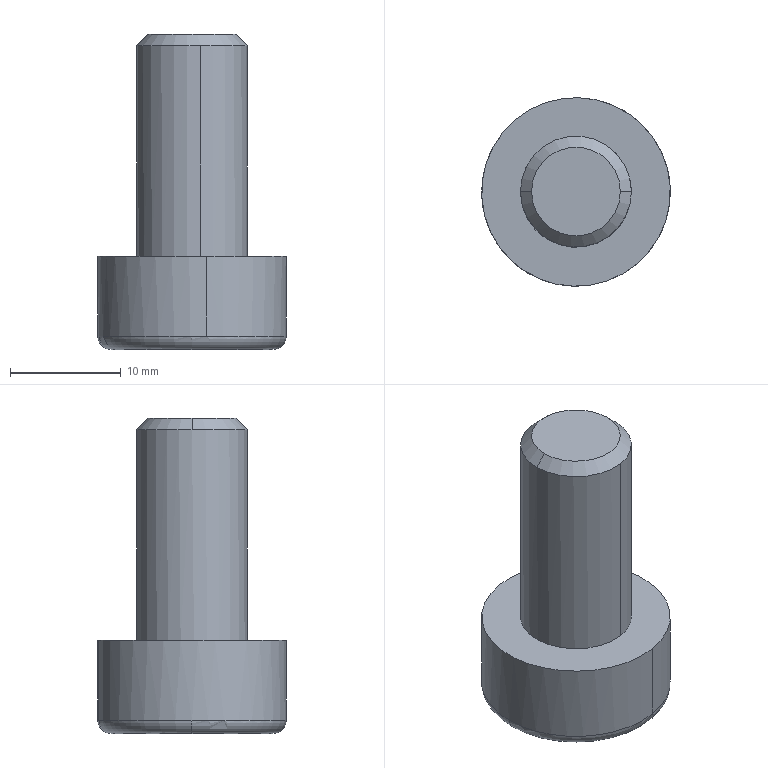Part | SolidWorks | features BaseBody 1 | 1 solid | 18 faces | box 17.001 x 17 x 28.402 mm | volume 3098 mm3 | plane 10 | cylinder 4 | cone 2 | torus 2 | commonest cylinder face diameters 10 x2 17 x2
STEP:
#1=CARTESIAN_POINT('',(410.058,334.317,39.477));
#2=VERTEX_POINT('',#1);
#3=CARTESIAN_POINT('',(402.058,334.317,39.476));
#4=VERTEX_POINT('',#3);
#5=CARTESIAN_POINT('',(406.058,334.317,39.477));
#6=DIRECTION('',(-0.0001435,-0.000000521,1.));
#7=DIRECTION('',(-1.,0.,-0.0001435));
#8=AXIS2_PLACEMENT_3D('',#5,#6,#7);
#9=CIRCLE('',#8,4.);
#10=EDGE_CURVE('',#2,#4,#9,.T.);
#11=ORIENTED_EDGE('',*,*,#10,.F.);
#12=CARTESIAN_POINT('',(411.058,334.317,38.477));
#13=VERTEX_POINT('',#12);
#14=CARTESIAN_POINT('',(410.558,334.317,38.977));
#15=DIRECTION('',(0.7072,0.000000369,-0.707));
#16=VECTOR('',#15,1000.);
#17=LINE('',#14,#16);
#18=EDGE_CURVE('',#2,#13,#17,.T.);
#19=ORIENTED_EDGE('',*,*,#18,.T.);
#20=CARTESIAN_POINT('',(405.284,339.257,38.477));
#21=VERTEX_POINT('',#20);
#22=CARTESIAN_POINT('',(406.058,334.317,38.477));
#23=DIRECTION('',(-0.0001435,-0.000000521,1.));
#24=DIRECTION('',(-0.1548,0.988,-0.00002169));
#25=AXIS2_PLACEMENT_3D('',#22,#23,#24);
#26=CIRCLE('',#25,5.);
#27=EDGE_CURVE('',#13,#21,#26,.T.);
#28=ORIENTED_EDGE('',*,*,#27,.T.);
#29=CARTESIAN_POINT('',(401.058,334.317,38.476));
#30=VERTEX_POINT('',#29);
#31=CARTESIAN_POINT('',(406.058,334.317,38.477));
#32=DIRECTION('',(-0.0001435,-0.000000521,1.));
#33=DIRECTION('',(-0.1548,0.988,-0.00002169));
#34=AXIS2_PLACEMENT_3D('',#31,#32,#33);
#35=CIRCLE('',#34,5.);
#36=EDGE_CURVE('',#21,#30,#35,.T.);
#37=ORIENTED_EDGE('',*,*,#36,.T.);
#38=CARTESIAN_POINT('',(401.558,334.317,38.976));
#39=DIRECTION('',(-0.707,0.000000369,-0.7072));
#40=VECTOR('',#39,1000.);
#41=LINE('',#38,#40);
#42=EDGE_CURVE('',#4,#30,#41,.T.);
#43=ORIENTED_EDGE('',*,*,#42,.F.);
#44=EDGE_LOOP('',(#11,#19,#28,#37,#43));
#45=FACE_OUTER_BOUND('',#44,.T.);
#46=CARTESIAN_POINT('',(406.058,334.317,38.977));
#47=DIRECTION('',(0.0001435,0.000000521,-1.));
#48=DIRECTION('',(-1.,0.,-0.0001435));
#49=AXIS2_PLACEMENT_3D('',#46,#47,#48);
#50=CONICAL_SURFACE('',#49,4.5,0.7854);
#51=ADVANCED_FACE('',(#45),#50,.T.);
#52=CARTESIAN_POINT('',(406.835,329.377,19.477));
#53=VERTEX_POINT('',#52);
#54=CARTESIAN_POINT('',(405.287,339.257,19.477));
#55=VERTEX_POINT('',#54);
#56=CARTESIAN_POINT('',(406.061,334.317,19.477));
#57=DIRECTION('',(0.0001435,0.000000521,-1.));
#58=DIRECTION('',(1.,0.,0.0001435));
#59=AXIS2_PLACEMENT_3D('',#56,#57,#58);
#60=CIRCLE('',#59,5.);
#61=EDGE_CURVE('',#53,#55,#60,.T.);
#62=ORIENTED_EDGE('',*,*,#61,.F.);
#63=CARTESIAN_POINT('',(406.832,329.377,38.477));
#64=VERTEX_POINT('',#63);
#65=CARTESIAN_POINT('',(406.832,329.377,41.277));
#66=DIRECTION('',(-0.0001435,-0.000000521,1.));
#67=VECTOR('',#66,1000.);
#68=LINE('',#65,#67);
#69=EDGE_CURVE('',#53,#64,#68,.T.);
#70=ORIENTED_EDGE('',*,*,#69,.T.);
#71=CARTESIAN_POINT('',(406.058,334.317,38.477));
#72=DIRECTION('',(-0.0001435,-0.000000521,1.));
#73=DIRECTION('',(-0.1548,0.988,-0.00002169));
#74=AXIS2_PLACEMENT_3D('',#71,#72,#73);
#75=CIRCLE('',#74,5.);
#76=EDGE_CURVE('',#30,#64,#75,.T.);
#77=ORIENTED_EDGE('',*,*,#76,.F.);
#78=ORIENTED_EDGE('',*,*,#36,.F.);
#79=CARTESIAN_POINT('',(405.284,339.257,41.277));
#80=DIRECTION('',(-0.0001435,-0.000000521,1.));
#81=VECTOR('',#80,1000.);
#82=LINE('',#79,#81);
#83=EDGE_CURVE('',#55,#21,#82,.T.);
#84=ORIENTED_EDGE('',*,*,#83,.F.);
#85=EDGE_LOOP('',(#62,#70,#77,#78,#84));
#86=FACE_OUTER_BOUND('',#85,.T.);
#87=CARTESIAN_POINT('',(406.058,334.317,41.277));
#88=DIRECTION('',(-0.0001435,-0.000000521,1.));
#89=DIRECTION('',(-0.1548,0.988,-0.00002169));
#90=AXIS2_PLACEMENT_3D('',#87,#88,#89);
#91=CYLINDRICAL_SURFACE('',#90,5.);
#92=ADVANCED_FACE('',(#86),#91,.T.);
#93=CARTESIAN_POINT('',(404.747,342.715,19.476));
#94=VERTEX_POINT('',#93);
#95=CARTESIAN_POINT('',(407.378,325.919,19.477));
#96=VERTEX_POINT('',#95);
#97=CARTESIAN_POINT('',(406.062,334.317,19.477));
#98=DIRECTION('',(-0.0001435,-0.000000521,1.));
#99=DIRECTION('',(-0.1548,0.988,-0.00002169));
#100=AXIS2_PLACEMENT_3D('',#97,#98,#99);
#101=CIRCLE('',#100,8.5);
#102=EDGE_CURVE('',#94,#96,#101,.T.);
#103=ORIENTED_EDGE('',*,*,#102,.F.);
#104=CARTESIAN_POINT('',(404.748,342.715,12.276));
#105=VERTEX_POINT('',#104);
#106=CARTESIAN_POINT('',(404.747,342.715,19.476));
#107=DIRECTION('',(0.0001435,0.000000521,-1.));
#108=VECTOR('',#107,1000.);
#109=LINE('',#106,#108);
#110=EDGE_CURVE('',#94,#105,#109,.T.);
#111=ORIENTED_EDGE('',*,*,#110,.T.);
#112=CARTESIAN_POINT('',(397.563,334.317,12.275));
#113=VERTEX_POINT('',#112);
#114=CARTESIAN_POINT('',(406.063,334.317,12.277));
#115=DIRECTION('',(0.0001435,0.000000521,-1.));
#116=DIRECTION('',(-0.1548,0.988,-0.00002169));
#117=AXIS2_PLACEMENT_3D('',#114,#115,#116);
#118=CIRCLE('',#117,8.5);
#119=EDGE_CURVE('',#113,#105,#118,.T.);
#120=ORIENTED_EDGE('',*,*,#119,.F.);
#121=CARTESIAN_POINT('',(407.379,325.919,12.277));
#122=VERTEX_POINT('',#121);
#123=CARTESIAN_POINT('',(406.063,334.317,12.277));
#124=DIRECTION('',(0.0001435,0.000000521,-1.));
#125=DIRECTION('',(-0.1548,0.988,-0.00002169));
#126=AXIS2_PLACEMENT_3D('',#123,#124,#125);
#127=CIRCLE('',#126,8.5);
#128=EDGE_CURVE('',#122,#113,#127,.T.);
#129=ORIENTED_EDGE('',*,*,#128,.F.);
#130=CARTESIAN_POINT('',(407.378,325.919,19.477));
#131=DIRECTION('',(0.0001435,0.000000521,-1.));
#132=VECTOR('',#131,1000.);
#133=LINE('',#130,#132);
#134=EDGE_CURVE('',#96,#122,#133,.T.);
#135=ORIENTED_EDGE('',*,*,#134,.F.);
#136=EDGE_LOOP('',(#103,#111,#120,#129,#135));
#137=FACE_OUTER_BOUND('',#136,.T.);
#138=CARTESIAN_POINT('',(406.062,334.317,19.477));
#139=DIRECTION('',(0.0001435,0.000000521,-1.));
#140=DIRECTION('',(0.1548,-0.988,0.00002169));
#141=AXIS2_PLACEMENT_3D('',#138,#139,#140);
#142=CYLINDRICAL_SURFACE('',#141,8.5);
#143=ADVANCED_FACE('',(#137),#142,.T.);
#144=ORIENTED_EDGE('',*,*,#119,.T.);
#145=CARTESIAN_POINT('',(414.563,334.317,12.278));
#146=VERTEX_POINT('',#145);
#147=CARTESIAN_POINT('',(406.063,334.317,12.277));
#148=DIRECTION('',(0.0001435,0.000000521,-1.));
#149=DIRECTION('',(-0.1548,0.988,-0.00002169));
#150=AXIS2_PLACEMENT_3D('',#147,#148,#149);
#151=CIRCLE('',#150,8.5);
#152=EDGE_CURVE('',#105,#146,#151,.T.);
#153=ORIENTED_EDGE('',*,*,#152,.T.);
#154=CARTESIAN_POINT('',(413.364,334.317,11.078));
#155=VERTEX_POINT('',#154);
#156=CARTESIAN_POINT('',(413.363,334.317,12.278));
#157=DIRECTION('',(0.,1.,0.000000521));
#158=DIRECTION('',(0.,-0.000000521,1.));
#159=AXIS2_PLACEMENT_3D('',#156,#157,#158);
#160=CIRCLE('',#159,1.2);
#161=EDGE_CURVE('',#146,#155,#160,.T.);
#162=ORIENTED_EDGE('',*,*,#161,.T.);
#163=CARTESIAN_POINT('',(398.764,334.317,11.076));
#164=VERTEX_POINT('',#163);
#165=CARTESIAN_POINT('',(406.064,334.317,11.077));
#166=DIRECTION('',(0.0001435,0.000000521,-1.));
#167=DIRECTION('',(-1.,0.,-0.0001435));
#168=AXIS2_PLACEMENT_3D('',#165,#166,#167);
#169=CIRCLE('',#168,7.3);
#170=EDGE_CURVE('',#164,#155,#169,.T.);
#171=ORIENTED_EDGE('',*,*,#170,.F.);
#172=CARTESIAN_POINT('',(398.763,334.317,12.276));
#173=DIRECTION('',(0.,-1.,-0.000000521));
#174=DIRECTION('',(0.,0.000000521,-1.));
#175=AXIS2_PLACEMENT_3D('',#172,#173,#174);
#176=CIRCLE('',#175,1.2);
#177=EDGE_CURVE('',#113,#164,#176,.T.);
#178=ORIENTED_EDGE('',*,*,#177,.F.);
#179=EDGE_LOOP('',(#144,#153,#162,#171,#178));
#180=FACE_OUTER_BOUND('',#179,.T.);
#181=CARTESIAN_POINT('',(406.063,334.317,12.277));
#182=DIRECTION('',(0.0001435,0.000000521,-1.));
#183=DIRECTION('',(-1.,0.,-0.0001435));
#184=AXIS2_PLACEMENT_3D('',#181,#182,#183);
#185=TOROIDAL_SURFACE('',#184,7.3,1.2);
#186=ADVANCED_FACE('',(#180),#185,.T.);
#187=CARTESIAN_POINT('',(410.797,335.039,17.077));
#188=VERTEX_POINT('',#187);
#189=CARTESIAN_POINT('',(409.094,330.624,17.077));
#190=VERTEX_POINT('',#189);
#191=CARTESIAN_POINT('',(410.797,335.039,17.077));
#192=DIRECTION('',(-0.3599,-0.933,-0.00005213));
#193=VECTOR('',#192,1000.);
#194=LINE('',#191,#193);
#195=EDGE_CURVE('',#188,#190,#194,.T.);
#196=ORIENTED_EDGE('',*,*,#195,.T.);
#197=CARTESIAN_POINT('',(404.419,329.891,17.076));
#198=VERTEX_POINT('',#197);
#199=CARTESIAN_POINT('',(409.094,330.624,17.077));
#200=DIRECTION('',(-0.988,-0.1548,-0.0001418));
#201=VECTOR('',#200,1000.);
#202=LINE('',#199,#201);
#203=EDGE_CURVE('',#190,#198,#202,.T.);
#204=ORIENTED_EDGE('',*,*,#203,.T.);
#205=CARTESIAN_POINT('',(401.447,333.574,17.076));
#206=VERTEX_POINT('',#205);
#207=CARTESIAN_POINT('',(404.419,329.891,17.076));
#208=DIRECTION('',(-0.628,0.7782,-0.0000897));
#209=VECTOR('',#208,1000.);
#210=LINE('',#207,#209);
#211=EDGE_CURVE('',#198,#206,#210,.T.);
#212=ORIENTED_EDGE('',*,*,#211,.T.);
#213=CARTESIAN_POINT('',(403.15,337.989,17.076));
#214=VERTEX_POINT('',#213);
#215=CARTESIAN_POINT('',(401.447,333.574,17.076));
#216=DIRECTION('',(0.3599,0.933,0.00005213));
#217=VECTOR('',#216,1000.);
#218=LINE('',#215,#217);
#219=EDGE_CURVE('',#206,#214,#218,.T.);
#220=ORIENTED_EDGE('',*,*,#219,.T.);
#221=CARTESIAN_POINT('',(407.825,338.721,17.077));
#222=VERTEX_POINT('',#221);
#223=CARTESIAN_POINT('',(403.15,337.989,17.076));
#224=DIRECTION('',(0.988,0.1548,0.0001418));
#225=VECTOR('',#224,1000.);
#226=LINE('',#223,#225);
#227=EDGE_CURVE('',#214,#222,#226,.T.);
#228=ORIENTED_EDGE('',*,*,#227,.T.);
#229=CARTESIAN_POINT('',(407.825,338.721,17.077));
#230=DIRECTION('',(0.628,-0.7782,0.0000897));
#231=VECTOR('',#230,1000.);
#232=LINE('',#229,#231);
#233=EDGE_CURVE('',#222,#188,#232,.T.);
#234=ORIENTED_EDGE('',*,*,#233,.T.);
#235=EDGE_LOOP('',(#196,#204,#212,#220,#228,#234));
#236=FACE_OUTER_BOUND('',#235,.T.);
#237=CARTESIAN_POINT('',(410.567,305.568,17.077));
#238=DIRECTION('',(0.0001435,0.000000521,-1.));
#239=DIRECTION('',(0.,-1.,-0.000000521));
#240=AXIS2_PLACEMENT_3D('',#237,#238,#239);
#241=PLANE('',#240);
#242=ADVANCED_FACE('',(#236),#241,.T.);
#243=CARTESIAN_POINT('',(409.095,330.624,11.077));
#244=VERTEX_POINT('',#243);
#245=CARTESIAN_POINT('',(409.094,330.624,17.077));
#246=DIRECTION('',(0.0001435,0.000000521,-1.));
#247=VECTOR('',#246,1000.);
#248=LINE('',#245,#247);
#249=EDGE_CURVE('',#190,#244,#248,.T.);
#250=ORIENTED_EDGE('',*,*,#249,.F.);
#251=ORIENTED_EDGE('',*,*,#195,.F.);
#252=CARTESIAN_POINT('',(410.798,335.039,11.077));
#253=VERTEX_POINT('',#252);
#254=CARTESIAN_POINT('',(410.797,335.039,17.077));
#255=DIRECTION('',(0.0001435,0.000000521,-1.));
#256=VECTOR('',#255,1000.);
#257=LINE('',#254,#256);
#258=EDGE_CURVE('',#188,#253,#257,.T.);
#259=ORIENTED_EDGE('',*,*,#258,.T.);
#260=CARTESIAN_POINT('',(409.095,330.624,11.077));
#261=DIRECTION('',(0.3599,0.933,0.00005213));
#262=VECTOR('',#261,1000.);
#263=LINE('',#260,#262);
#264=EDGE_CURVE('',#244,#253,#263,.T.);
#265=ORIENTED_EDGE('',*,*,#264,.F.);
#266=EDGE_LOOP('',(#250,#251,#259,#265));
#267=FACE_OUTER_BOUND('',#266,.T.);
#268=CARTESIAN_POINT('',(410.485,334.231,17.077));
#269=DIRECTION('',(0.933,-0.3599,0.0001337));
#270=DIRECTION('',(0.,-0.0003714,-1.));
#271=AXIS2_PLACEMENT_3D('',#268,#269,#270);
#272=PLANE('',#271);
#273=ADVANCED_FACE('',(#267),#272,.F.);
#274=CARTESIAN_POINT('',(404.42,329.891,11.076));
#275=VERTEX_POINT('',#274);
#276=CARTESIAN_POINT('',(404.419,329.891,17.076));
#277=DIRECTION('',(0.0001435,0.000000521,-1.));
#278=VECTOR('',#277,1000.);
#279=LINE('',#276,#278);
#280=EDGE_CURVE('',#198,#275,#279,.T.);
#281=ORIENTED_EDGE('',*,*,#280,.F.);
#282=ORIENTED_EDGE('',*,*,#203,.F.);
#283=ORIENTED_EDGE('',*,*,#249,.T.);
#284=CARTESIAN_POINT('',(404.42,329.891,11.076));
#285=DIRECTION('',(0.988,0.1548,0.0001418));
#286=VECTOR('',#285,1000.);
#287=LINE('',#284,#286);
#288=EDGE_CURVE('',#275,#244,#287,.T.);
#289=ORIENTED_EDGE('',*,*,#288,.F.);
#290=EDGE_LOOP('',(#281,#282,#283,#289));
#291=FACE_OUTER_BOUND('',#290,.T.);
#292=CARTESIAN_POINT('',(408.238,330.49,17.077));
#293=DIRECTION('',(0.1548,-0.988,0.00002169));
#294=DIRECTION('',(0.,-0.00002196,-1.));
#295=AXIS2_PLACEMENT_3D('',#292,#293,#294);
#296=PLANE('',#295);
#297=ADVANCED_FACE('',(#291),#296,.F.);
#298=CARTESIAN_POINT('',(401.448,333.574,11.076));
#299=VERTEX_POINT('',#298);
#300=CARTESIAN_POINT('',(401.447,333.574,17.076));
#301=DIRECTION('',(0.0001435,0.000000521,-1.));
#302=VECTOR('',#301,1000.);
#303=LINE('',#300,#302);
#304=EDGE_CURVE('',#206,#299,#303,.T.);
#305=ORIENTED_EDGE('',*,*,#304,.F.);
#306=ORIENTED_EDGE('',*,*,#211,.F.);
#307=ORIENTED_EDGE('',*,*,#280,.T.);
#308=CARTESIAN_POINT('',(401.448,333.574,11.076));
#309=DIRECTION('',(0.628,-0.7782,0.0000897));
#310=VECTOR('',#309,1000.);
#311=LINE('',#308,#310);
#312=EDGE_CURVE('',#299,#275,#311,.T.);
#313=ORIENTED_EDGE('',*,*,#312,.F.);
#314=EDGE_LOOP('',(#305,#306,#307,#313));
#315=FACE_OUTER_BOUND('',#314,.T.);
#316=CARTESIAN_POINT('',(403.875,330.565,17.076));
#317=DIRECTION('',(-0.7782,-0.628,-0.000112));
#318=DIRECTION('',(-0.628,0.7782,0.));
#319=AXIS2_PLACEMENT_3D('',#316,#317,#318);
#320=PLANE('',#319);
#321=ADVANCED_FACE('',(#315),#320,.F.);
#322=CARTESIAN_POINT('',(403.151,337.989,11.076));
#323=VERTEX_POINT('',#322);
#324=CARTESIAN_POINT('',(403.15,337.989,17.076));
#325=DIRECTION('',(0.0001435,0.000000521,-1.));
#326=VECTOR('',#325,1000.);
#327=LINE('',#324,#326);
#328=EDGE_CURVE('',#214,#323,#327,.T.);
#329=ORIENTED_EDGE('',*,*,#328,.F.);
#330=ORIENTED_EDGE('',*,*,#219,.F.);
#331=ORIENTED_EDGE('',*,*,#304,.T.);
#332=CARTESIAN_POINT('',(403.151,337.989,11.076));
#333=DIRECTION('',(-0.3599,-0.933,-0.00005213));
#334=VECTOR('',#333,1000.);
#335=LINE('',#332,#334);
#336=EDGE_CURVE('',#323,#299,#335,.T.);
#337=ORIENTED_EDGE('',*,*,#336,.F.);
#338=EDGE_LOOP('',(#329,#330,#331,#337));
#339=FACE_OUTER_BOUND('',#338,.T.);
#340=CARTESIAN_POINT('',(401.759,334.382,17.076));
#341=DIRECTION('',(-0.933,0.3599,-0.0001337));
#342=DIRECTION('',(-0.0001433,0.,1.));
#343=AXIS2_PLACEMENT_3D('',#340,#341,#342);
#344=PLANE('',#343);
#345=ADVANCED_FACE('',(#339),#344,.F.);
#346=CARTESIAN_POINT('',(407.826,338.721,11.077));
#347=VERTEX_POINT('',#346);
#348=CARTESIAN_POINT('',(407.825,338.721,17.077));
#349=DIRECTION('',(0.0001435,0.000000521,-1.));
#350=VECTOR('',#349,1000.);
#351=LINE('',#348,#350);
#352=EDGE_CURVE('',#222,#347,#351,.T.);
#353=ORIENTED_EDGE('',*,*,#352,.F.);
#354=ORIENTED_EDGE('',*,*,#227,.F.);
#355=ORIENTED_EDGE('',*,*,#328,.T.);
#356=CARTESIAN_POINT('',(407.826,338.721,11.077));
#357=DIRECTION('',(-0.988,-0.1548,-0.0001418));
#358=VECTOR('',#357,1000.);
#359=LINE('',#356,#358);
#360=EDGE_CURVE('',#347,#323,#359,.T.);
#361=ORIENTED_EDGE('',*,*,#360,.F.);
#362=EDGE_LOOP('',(#353,#354,#355,#361));
#363=FACE_OUTER_BOUND('',#362,.T.);
#364=CARTESIAN_POINT('',(404.006,338.123,17.076));
#365=DIRECTION('',(-0.1548,0.988,-0.00002169));
#366=DIRECTION('',(-0.0001401,0.,1.));
#367=AXIS2_PLACEMENT_3D('',#364,#365,#366);
#368=PLANE('',#367);
#369=ADVANCED_FACE('',(#363),#368,.F.);
#370=ORIENTED_EDGE('',*,*,#258,.F.);
#371=ORIENTED_EDGE('',*,*,#233,.F.);
#372=ORIENTED_EDGE('',*,*,#352,.T.);
#373=CARTESIAN_POINT('',(410.798,335.039,11.077));
#374=DIRECTION('',(-0.628,0.7782,-0.0000897));
#375=VECTOR('',#374,1000.);
#376=LINE('',#373,#375);
#377=EDGE_CURVE('',#253,#347,#376,.T.);
#378=ORIENTED_EDGE('',*,*,#377,.F.);
#379=EDGE_LOOP('',(#370,#371,#372,#378));
#380=FACE_OUTER_BOUND('',#379,.T.);
#381=CARTESIAN_POINT('',(408.369,338.047,17.077));
#382=DIRECTION('',(0.7782,0.628,0.000112));
#383=DIRECTION('',(0.,0.0001783,-1.));
#384=AXIS2_PLACEMENT_3D('',#381,#382,#383);
#385=PLANE('',#384);
#386=ADVANCED_FACE('',(#380),#385,.F.);
#387=ORIENTED_EDGE('',*,*,#360,.T.);
#388=ORIENTED_EDGE('',*,*,#336,.T.);
#389=ORIENTED_EDGE('',*,*,#312,.T.);
#390=ORIENTED_EDGE('',*,*,#288,.T.);
#391=ORIENTED_EDGE('',*,*,#264,.T.);
#392=ORIENTED_EDGE('',*,*,#377,.T.);
#393=EDGE_LOOP('',(#387,#388,#389,#390,#391,#392));
#394=FACE_BOUND('',#393,.T.);
#395=ORIENTED_EDGE('',*,*,#170,.T.);
#396=CARTESIAN_POINT('',(406.064,334.317,11.077));
#397=DIRECTION('',(0.0001435,0.000000521,-1.));
#398=DIRECTION('',(-1.,0.,-0.0001435));
#399=AXIS2_PLACEMENT_3D('',#396,#397,#398);
#400=CIRCLE('',#399,7.3);
#401=EDGE_CURVE('',#155,#164,#400,.T.);
#402=ORIENTED_EDGE('',*,*,#401,.T.);
#403=EDGE_LOOP('',(#395,#402));
#404=FACE_OUTER_BOUND('',#403,.T.);
#405=CARTESIAN_POINT('',(406.064,334.317,11.077));
#406=DIRECTION('',(0.0001435,0.000000521,-1.));
#407=DIRECTION('',(0.,-1.,-0.000000521));
#408=AXIS2_PLACEMENT_3D('',#405,#406,#407);
#409=PLANE('',#408);
#410=ADVANCED_FACE('',(#394,#404),#409,.T.);
#411=ORIENTED_EDGE('',*,*,#161,.F.);
#412=CARTESIAN_POINT('',(406.063,334.317,12.277));
#413=DIRECTION('',(0.0001435,0.000000521,-1.));
#414=DIRECTION('',(-0.1548,0.988,-0.00002169));
#415=AXIS2_PLACEMENT_3D('',#412,#413,#414);
#416=CIRCLE('',#415,8.5);
#417=EDGE_CURVE('',#146,#122,#416,.T.);
#418=ORIENTED_EDGE('',*,*,#417,.T.);
#419=ORIENTED_EDGE('',*,*,#128,.T.);
#420=ORIENTED_EDGE('',*,*,#177,.T.);
#421=ORIENTED_EDGE('',*,*,#401,.F.);
#422=EDGE_LOOP('',(#411,#418,#419,#420,#421));
#423=FACE_OUTER_BOUND('',#422,.T.);
#424=CARTESIAN_POINT('',(406.063,334.317,12.277));
#425=DIRECTION('',(0.0001435,0.000000521,-1.));
#426=DIRECTION('',(-1.,0.,-0.0001435));
#427=AXIS2_PLACEMENT_3D('',#424,#425,#426);
#428=TOROIDAL_SURFACE('',#427,7.3,1.2);
#429=ADVANCED_FACE('',(#423),#428,.T.);
#430=ORIENTED_EDGE('',*,*,#110,.F.);
#431=CARTESIAN_POINT('',(406.062,334.317,19.477));
#432=DIRECTION('',(-0.0001435,-0.000000521,1.));
#433=DIRECTION('',(-0.1548,0.988,-0.00002169));
#434=AXIS2_PLACEMENT_3D('',#431,#432,#433);
#435=CIRCLE('',#434,8.5);
#436=EDGE_CURVE('',#96,#94,#435,.T.);
#437=ORIENTED_EDGE('',*,*,#436,.F.);
#438=ORIENTED_EDGE('',*,*,#134,.T.);
#439=ORIENTED_EDGE('',*,*,#417,.F.);
#440=ORIENTED_EDGE('',*,*,#152,.F.);
#441=EDGE_LOOP('',(#430,#437,#438,#439,#440));
#442=FACE_OUTER_BOUND('',#441,.T.);
#443=CARTESIAN_POINT('',(406.062,334.317,19.477));
#444=DIRECTION('',(0.0001435,0.000000521,-1.));
#445=DIRECTION('',(0.1548,-0.988,0.00002169));
#446=AXIS2_PLACEMENT_3D('',#443,#444,#445);
#447=CYLINDRICAL_SURFACE('',#446,8.5);
#448=ADVANCED_FACE('',(#442),#447,.T.);
#449=CARTESIAN_POINT('',(406.061,334.317,19.477));
#450=DIRECTION('',(0.0001435,0.000000521,-1.));
#451=DIRECTION('',(1.,0.,0.0001435));
#452=AXIS2_PLACEMENT_3D('',#449,#450,#451);
#453=CIRCLE('',#452,5.);
#454=EDGE_CURVE('',#55,#53,#453,.T.);
#455=ORIENTED_EDGE('',*,*,#454,.T.);
#456=ORIENTED_EDGE('',*,*,#61,.T.);
#457=EDGE_LOOP('',(#455,#456));
#458=FACE_BOUND('',#457,.T.);
#459=ORIENTED_EDGE('',*,*,#436,.T.);
#460=ORIENTED_EDGE('',*,*,#102,.T.);
#461=EDGE_LOOP('',(#459,#460));
#462=FACE_OUTER_BOUND('',#461,.T.);
#463=CARTESIAN_POINT('',(406.062,334.317,19.477));
#464=DIRECTION('',(-0.0001435,-0.000000521,1.));
#465=DIRECTION('',(-0.003633,1.,0.));
#466=AXIS2_PLACEMENT_3D('',#463,#464,#465);
#467=PLANE('',#466);
#468=ADVANCED_FACE('',(#458,#462),#467,.T.);
#469=ORIENTED_EDGE('',*,*,#69,.F.);
#470=ORIENTED_EDGE('',*,*,#454,.F.);
#471=ORIENTED_EDGE('',*,*,#83,.T.);
#472=ORIENTED_EDGE('',*,*,#27,.F.);
#473=CARTESIAN_POINT('',(406.058,334.317,38.477));
#474=DIRECTION('',(-0.0001435,-0.000000521,1.));
#475=DIRECTION('',(-0.1548,0.988,-0.00002169));
#476=AXIS2_PLACEMENT_3D('',#473,#474,#475);
#477=CIRCLE('',#476,5.);
#478=EDGE_CURVE('',#64,#13,#477,.T.);
#479=ORIENTED_EDGE('',*,*,#478,.F.);
#480=EDGE_LOOP('',(#469,#470,#471,#472,#479));
#481=FACE_OUTER_BOUND('',#480,.T.);
#482=CARTESIAN_POINT('',(406.058,334.317,41.277));
#483=DIRECTION('',(-0.0001435,-0.000000521,1.));
#484=DIRECTION('',(-0.1548,0.988,-0.00002169));
#485=AXIS2_PLACEMENT_3D('',#482,#483,#484);
#486=CYLINDRICAL_SURFACE('',#485,5.);
#487=ADVANCED_FACE('',(#481),#486,.T.);
#488=ORIENTED_EDGE('',*,*,#18,.F.);
#489=CARTESIAN_POINT('',(406.058,334.317,39.477));
#490=DIRECTION('',(-0.0001435,-0.000000521,1.));
#491=DIRECTION('',(-1.,0.,-0.0001435));
#492=AXIS2_PLACEMENT_3D('',#489,#490,#491);
#493=CIRCLE('',#492,4.);
#494=EDGE_CURVE('',#4,#2,#493,.T.);
#495=ORIENTED_EDGE('',*,*,#494,.F.);
#496=ORIENTED_EDGE('',*,*,#42,.T.);
#497=ORIENTED_EDGE('',*,*,#76,.T.);
#498=ORIENTED_EDGE('',*,*,#478,.T.);
#499=EDGE_LOOP('',(#488,#495,#496,#497,#498));
#500=FACE_OUTER_BOUND('',#499,.T.);
#501=CARTESIAN_POINT('',(406.058,334.317,38.977));
#502=DIRECTION('',(0.0001435,0.000000521,-1.));
#503=DIRECTION('',(-1.,0.,-0.0001435));
#504=AXIS2_PLACEMENT_3D('',#501,#502,#503);
#505=CONICAL_SURFACE('',#504,4.5,0.7854);
#506=ADVANCED_FACE('',(#500),#505,.T.);
#507=ORIENTED_EDGE('',*,*,#494,.T.);
#508=ORIENTED_EDGE('',*,*,#10,.T.);
#509=EDGE_LOOP('',(#507,#508));
#510=FACE_OUTER_BOUND('',#509,.T.);
#511=CARTESIAN_POINT('',(406.06,334.317,39.477));
#512=DIRECTION('',(-0.0001435,-0.000000521,1.));
#513=DIRECTION('',(-0.003633,1.,0.));
#514=AXIS2_PLACEMENT_3D('',#511,#512,#513);
#515=PLANE('',#514);
#516=ADVANCED_FACE('',(#510),#515,.T.);
#517=CLOSED_SHELL('',(#51,#92,#143,#186,#242,#273,#297,#321,#345,#369,#386,#410,#429,#448,#468,#487,#506,#516));
#518=MANIFOLD_SOLID_BREP('',#517);
#519=CARTESIAN_POINT('',(0.,0.,0.));
#520=DIRECTION('',(0.,0.,1.));
#521=DIRECTION('',(1.,0.,0.));
#522=AXIS2_PLACEMENT_3D('',#519,#520,#521);
#523=(LENGTH_UNIT()NAMED_UNIT(*)SI_UNIT(.MILLI.,.METRE.));
#524=UNCERTAINTY_MEASURE_WITH_UNIT(LENGTH_MEASURE(0.00001),#523,'','');
#525=(NAMED_UNIT(*)PLANE_ANGLE_UNIT()SI_UNIT($,.RADIAN.));
#526=(NAMED_UNIT(*)SI_UNIT($,.STERADIAN.)SOLID_ANGLE_UNIT());
#527=(GEOMETRIC_REPRESENTATION_CONTEXT(3)GLOBAL_UNCERTAINTY_ASSIGNED_CONTEXT((#524))GLOBAL_UNIT_ASSIGNED_CONTEXT((#523,#525,#526))REPRESENTATION_CONTEXT('',''));
#528=ADVANCED_BREP_SHAPE_REPRESENTATION('',(#518,#522),#527);